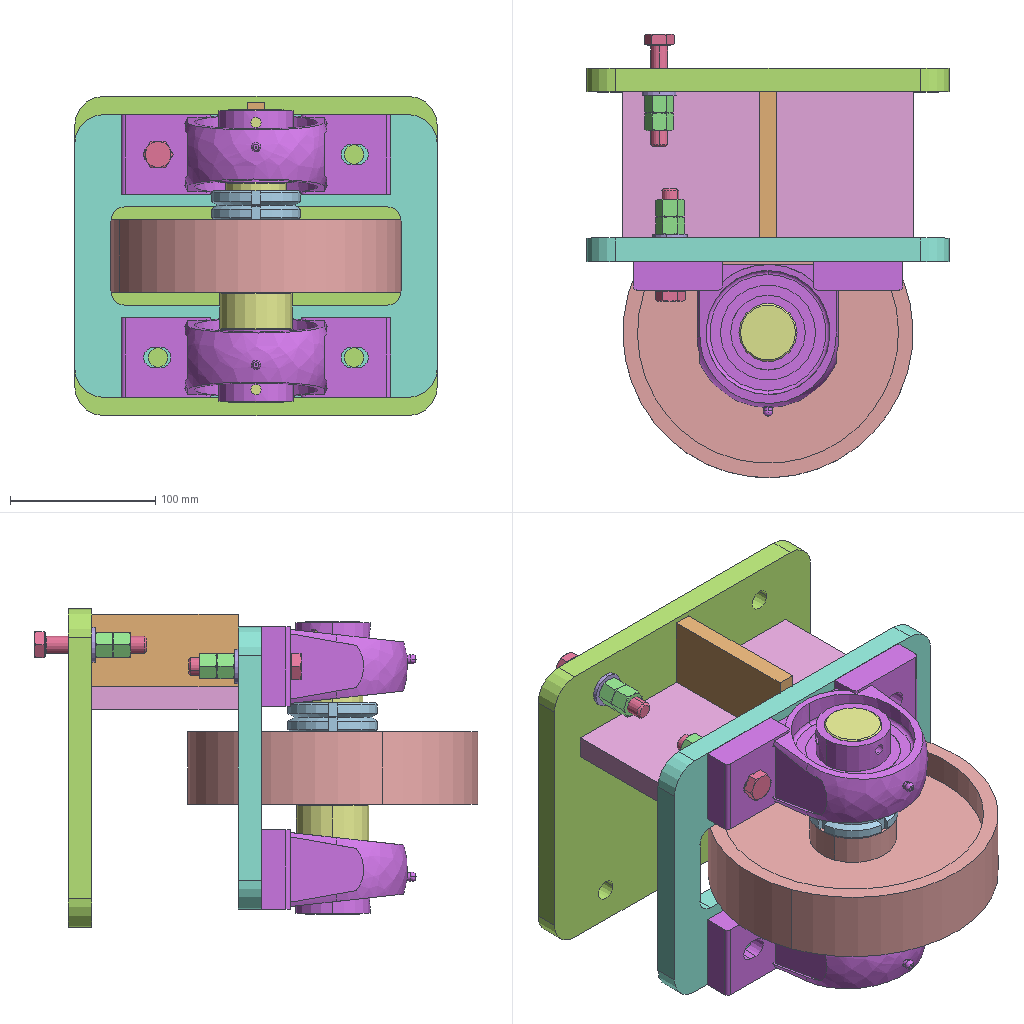Assembly | SolidWorks | 13 different items | 20 placed | box 250 x 306 x 220 mm
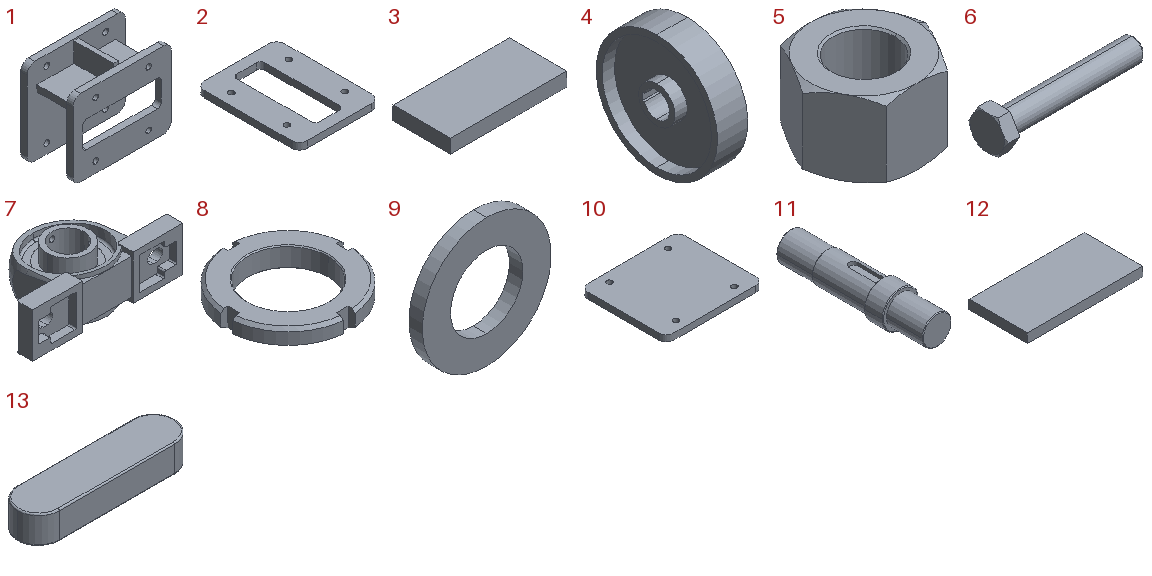Parts list (item | name | quantity | parent item | size | volume | features):
1 | (subassembly) | x1 | - | 250 x 133 x 220 mm | 1797573 mm3 | -
2 | - | x1 | in 1 | 195 x 250 x 16 mm | 549119 mm3 | features Fillet 2, Chamfer 1, Extrusion 1, HoleWzd 1
3 | - | x1 | in 1 | 101 x 50 x 12 mm | 60600 mm3 | features Extrusion 1
4 | - | x1 | - | 50 x 200 x 200 mm | 594592 mm3 | features ICE 1, Revolution 1
5 | - | x4 | - | 19.9 x 17.234 x 12.2 mm | 2145 mm3 | features Cut 2, Chamfer 1, Extrusion 1
6 | - | x2 | - | 77.5 x 20.785 x 18 mm | 9947 mm3 | features RevCut 4, Revolution 2, Chamfer 1, Extrusion 1, LPattern 1
7 | - | x2 | - | 186 x 106.8 x 57.7 mm | 279855 mm3 | features Revolution 5, Cut 3, Boss 2, CirPattern 2, ICE 2, RevCut 2, Extrusion 1, RefAxis 1, SweepCut 1
8 | - | x2 | - | 61.709 x 61.709 x 10 mm | 15331 mm3 | features Chamfer 3, CirPattern 1, Cut 1, Extrusion 1
9 | - | x2 | - | 24 x 2.5 x 24 mm | 773.126 mm3 | features Revolution 1
10 | - | x1 | in 1 | 250 x 220 x 16 mm | 864654 mm3 | features Chamfer 1, Extrusion 1, Fillet 1, HoleWzd 1
11 | - | x1 | - | 50 x 202 x 50 mm | 279258 mm3 | features Chamfer 1, ICE 1, Revolution 1
12 | - | x1 | in 1 | 200 x 101 x 16 mm | 323200 mm3 | features Extrusion 1
13 | - | x1 | - | 45 x 12 x 8 mm | 4066 mm3 | features Extrusion 1, Fillet 1
Mates (type | each side: item.copy, entity, surface, feature):
In the top assembly
Coincident | 1.1 plane | assembly plane | 3 times
Coincident | 2.1 face plane Boss-Extrude1 | 7.1 face plane Boss-Extrude1
Coincident | 7.1 plane | assembly plane
Coincident | 2.1 face plane Boss-Extrude1 | 7.2 face plane Boss-Extrude1
Slot | 2.1 face cylinder Ø13.5 Hole1 | 7.1 face plane Cut-Extrude3
Concentric | 7.1 face cylinder Boss-Revolve5 | 7.2 face cylinder Boss-Revolve5
Slot | 7.2 face plane Cut-Extrude3 | 2.1 face cylinder Ø13.5 Hole1
Concentric | 11.1 face cylinder Revolve1 | 7.2 face cylinder Boss-Revolve5
Coincident | 11.1 face plane Revolve1 | 7.1 face plane Boss-Revolve5
Concentric | 5.1 face cylinder Boss-Extrude | 5.2 face cylinder Boss-Extrude
Coincident | 5.1 face plane Boss-Extrude | 5.2 face plane Boss-Extrude | 2 times
Concentric | 6.1 face cylinder Boss-Revolve1 | 5.2 face cylinder Boss-Extrude
Concentric | 9.1 face cylinder Boss-Revolve | 6.1 face cylinder Boss-Revolve1
Coincident | 5.1 face plane Boss-Extrude | 9.1 face plane Boss-Revolve
Parallel | 5.1 face plane Boss-Extrude | 6.1 face plane Boss-Extrude
Concentric | 10.1 face cylinder Ø14 Hole1 | 6.1 face cylinder Boss-Revolve1
Coincident | 10.1 face plane Boss-Extrude1 | 9.1 face plane Boss-Revolve
Coincident | 5.3 face plane Boss-Extrude | 5.4 face plane Boss-Extrude | 2 times
Coincident | 5.4 face plane Boss-Extrude | 9.2 face plane Boss-Revolve
Concentric | 6.2 face cylinder Boss-Revolve1 | 9.2 face cylinder Boss-Revolve
Concentric | 6.2 face cylinder Boss-Revolve1 | 5.3 face cylinder Boss-Extrude
Concentric | 5.3 face cylinder Boss-Extrude | 5.4 face cylinder Boss-Extrude
Parallel | 6.2 face plane Boss-Extrude | 5.4 face plane Boss-Extrude
Concentric | 2.1 face cylinder Ø13.5 Hole1 | 6.2 face cylinder Boss-Revolve1
Coincident | 7.2 face plane Boss-Extrude1 | 6.2 face plane Boss-Extrude
Coincident | 2.1 face plane Boss-Extrude1 | 9.2 face plane Boss-Revolve
Coincident | 11.1 face plane Cut-Extrude1 | 13.1 face plane Boss-Extrude
Concentric | 11.1 face cylinder Cut-Extrude1 | 13.1 face cylinder Boss-Extrude
Parallel | 11.1 face plane Cut-Extrude1 | 13.1 face plane Boss-Extrude
Concentric | 11.1 face cylinder Revolve1 | 4.1 face cylinder Revolve1
Coincident | 11.1 face plane Revolve1 | 4.1 face plane Revolve1
Concentric | 8.1 face cylinder Boss-Extrude | 8.2 face cylinder Boss-Extrude
Coincident | 8.1 face plane Boss-Extrude | 8.2 face plane Boss-Extrude
Concentric | 11.1 face cylinder Revolve1 | 8.1 face cylinder Boss-Extrude
Coincident | 4.1 face plane Revolve1 | 8.2 face plane Boss-Extrude
Coincident | 8.1 face plane CirPattern1 | 8.2 face plane CirPattern1
Parallel | 2.1 face plane Boss-Extrude1 | 8.2 face plane CirPattern1
Parallel | 10.1 face plane Boss-Extrude1 | 6.1 face plane Boss-Extrude
Parallel | 5.3 face plane Boss-Extrude | 2.1 face plane Boss-Extrude1
Parallel | 11.1 plane | assembly plane
DistanceDim | 6.1 face plane Boss-Extrude | 10.1 face plane Boss-Extrude1
In subassembly 1
Coincident | 2.2 face plane Boss-Extrude1 | 1.2 plane
Coincident | 2.2 plane | 1.2 plane | 2 times
DistanceDim | 10.2 face plane Boss-Extrude1 | 2.2 face plane Boss-Extrude1
Width | 2.2 face plane Boss-Extrude1 | 2.2 face plane Boss-Extrude1 | 10.2 face plane Boss-Extrude1 | 10.2 face plane Boss-Extrude1
Width | 10.2 face plane Boss-Extrude1 | 10.2 face plane Boss-Extrude1 | 2.2 face plane Boss-Extrude1 | 2.2 face plane Boss-Extrude1
Coincident | 2.2 face plane Boss-Extrude1 | 12.1 face plane Boss-Extrude1
Coincident | 2.2 face plane Boss-Extrude1 | 3.1 face plane Boss-Extrude1
Coincident | 12.1 face plane Boss-Extrude1 | 3.1 face plane Boss-Extrude1
Width | 12.1 face plane Boss-Extrude1 | 12.1 face plane Boss-Extrude1 | 2.2 face plane Boss-Extrude1 | 2.2 face plane Boss-Extrude1
Width | 3.1 face plane Boss-Extrude1 | 3.1 face plane Boss-Extrude1 | 12.1 face plane Boss-Extrude1 | 12.1 face plane Boss-Extrude1